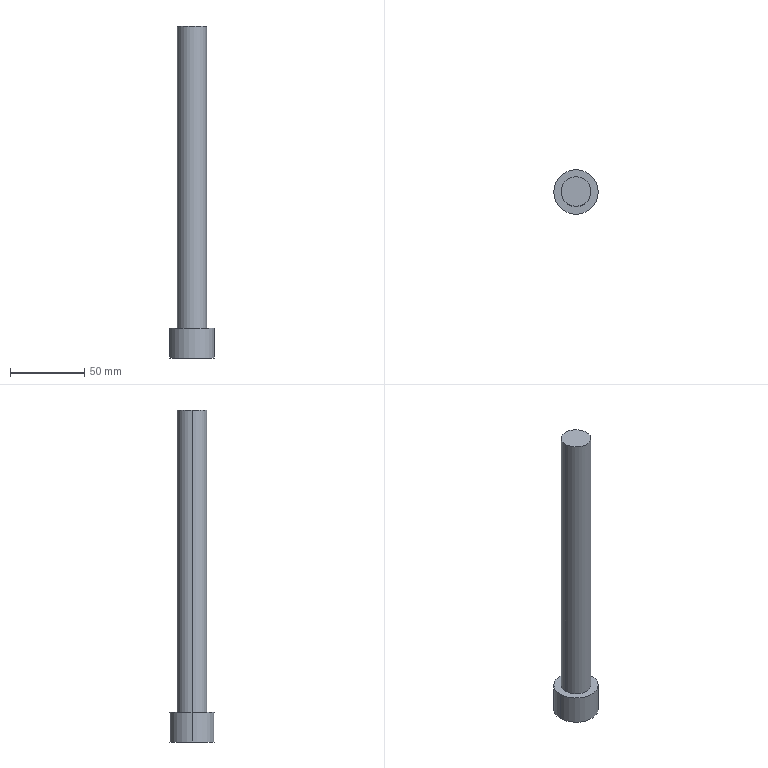Part | Creo | 1 solid | 14 faces | box 30 x 30 x 224 mm | volume 75420 mm3 | plane 10 | cylinder 4 | commonest cylinder face diameters 20 x2 30 x2
STEP:
#1=CARTESIAN_POINT('',(-235.,225.,-334.5));
#2=VERTEX_POINT('',#1);
#3=CARTESIAN_POINT('',(-265.,225.,-334.5));
#4=VERTEX_POINT('',#3);
#5=CARTESIAN_POINT('',(-250.,225.,-334.5));
#6=DIRECTION('',(0.,0.,-1.));
#7=DIRECTION('',(1.,0.,0.));
#8=AXIS2_PLACEMENT_3D('',#5,#6,#7);
#9=CIRCLE('',#8,15.);
#10=EDGE_CURVE('',#2,#4,#9,.T.);
#11=ORIENTED_EDGE('',*,*,#10,.F.);
#12=CARTESIAN_POINT('',(-250.,225.,-334.5));
#13=DIRECTION('',(0.,0.,-1.));
#14=DIRECTION('',(-1.,0.,0.));
#15=AXIS2_PLACEMENT_3D('',#12,#13,#14);
#16=CIRCLE('',#15,15.);
#17=EDGE_CURVE('',#4,#2,#16,.T.);
#18=ORIENTED_EDGE('',*,*,#17,.F.);
#19=EDGE_LOOP('',(#11,#18));
#20=FACE_OUTER_BOUND('',#19,.F.);
#21=CARTESIAN_POINT('',(-259.,219.804,-334.5));
#22=VERTEX_POINT('',#21);
#23=CARTESIAN_POINT('',(-250.,214.608,-334.5));
#24=VERTEX_POINT('',#23);
#25=CARTESIAN_POINT('',(-259.,219.804,-334.5));
#26=DIRECTION('',(0.866,-0.5,0.));
#27=VECTOR('',#26,10.392);
#28=LINE('',#25,#27);
#29=EDGE_CURVE('',#22,#24,#28,.T.);
#30=ORIENTED_EDGE('',*,*,#29,.F.);
#31=CARTESIAN_POINT('',(-259.,230.196,-334.5));
#32=VERTEX_POINT('',#31);
#33=CARTESIAN_POINT('',(-259.,219.804,-334.5));
#34=DIRECTION('',(0.,1.,0.));
#35=VECTOR('',#34,10.392);
#36=LINE('',#33,#35);
#37=EDGE_CURVE('',#22,#32,#36,.T.);
#38=ORIENTED_EDGE('',*,*,#37,.T.);
#39=CARTESIAN_POINT('',(-250.,235.392,-334.5));
#40=VERTEX_POINT('',#39);
#41=CARTESIAN_POINT('',(-250.,235.392,-334.5));
#42=DIRECTION('',(-0.866,-0.5,0.));
#43=VECTOR('',#42,10.392);
#44=LINE('',#41,#43);
#45=EDGE_CURVE('',#40,#32,#44,.T.);
#46=ORIENTED_EDGE('',*,*,#45,.F.);
#47=CARTESIAN_POINT('',(-241.,230.196,-334.5));
#48=VERTEX_POINT('',#47);
#49=CARTESIAN_POINT('',(-241.,230.196,-334.5));
#50=DIRECTION('',(-0.866,0.5,0.));
#51=VECTOR('',#50,10.392);
#52=LINE('',#49,#51);
#53=EDGE_CURVE('',#48,#40,#52,.T.);
#54=ORIENTED_EDGE('',*,*,#53,.F.);
#55=CARTESIAN_POINT('',(-241.,219.804,-334.5));
#56=VERTEX_POINT('',#55);
#57=CARTESIAN_POINT('',(-241.,230.196,-334.5));
#58=DIRECTION('',(0.,-1.,0.));
#59=VECTOR('',#58,10.392);
#60=LINE('',#57,#59);
#61=EDGE_CURVE('',#48,#56,#60,.T.);
#62=ORIENTED_EDGE('',*,*,#61,.T.);
#63=CARTESIAN_POINT('',(-250.,214.608,-334.5));
#64=DIRECTION('',(0.866,0.5,0.));
#65=VECTOR('',#64,10.392);
#66=LINE('',#63,#65);
#67=EDGE_CURVE('',#24,#56,#66,.T.);
#68=ORIENTED_EDGE('',*,*,#67,.F.);
#69=EDGE_LOOP('',(#30,#38,#46,#54,#62,#68));
#70=FACE_BOUND('',#69,.F.);
#71=CARTESIAN_POINT('',(-250.,225.,-334.5));
#72=DIRECTION('',(0.,0.,-1.));
#73=DIRECTION('',(-1.,0.,0.));
#74=AXIS2_PLACEMENT_3D('',#71,#72,#73);
#75=PLANE('',#74);
#76=ADVANCED_FACE('',(#20,#70),#75,.T.);
#77=CARTESIAN_POINT('',(-265.,225.,-314.5));
#78=VERTEX_POINT('',#77);
#79=CARTESIAN_POINT('',(-235.,225.,-314.5));
#80=VERTEX_POINT('',#79);
#81=CARTESIAN_POINT('',(-250.,225.,-314.5));
#82=DIRECTION('',(0.,0.,1.));
#83=DIRECTION('',(-1.,0.,0.));
#84=AXIS2_PLACEMENT_3D('',#81,#82,#83);
#85=CIRCLE('',#84,15.);
#86=EDGE_CURVE('',#78,#80,#85,.T.);
#87=ORIENTED_EDGE('',*,*,#86,.T.);
#88=CARTESIAN_POINT('',(-235.,225.,-334.5));
#89=DIRECTION('',(0.,0.,1.));
#90=VECTOR('',#89,20.);
#91=LINE('',#88,#90);
#92=EDGE_CURVE('',#2,#80,#91,.T.);
#93=ORIENTED_EDGE('',*,*,#92,.F.);
#94=ORIENTED_EDGE('',*,*,#10,.T.);
#95=CARTESIAN_POINT('',(-265.,225.,-334.5));
#96=DIRECTION('',(0.,0.,1.));
#97=VECTOR('',#96,20.);
#98=LINE('',#95,#97);
#99=EDGE_CURVE('',#4,#78,#98,.T.);
#100=ORIENTED_EDGE('',*,*,#99,.T.);
#101=EDGE_LOOP('',(#87,#93,#94,#100));
#102=FACE_OUTER_BOUND('',#101,.F.);
#103=CARTESIAN_POINT('',(-250.,225.,-334.5));
#104=DIRECTION('',(0.,0.,1.));
#105=DIRECTION('',(1.,0.,0.));
#106=AXIS2_PLACEMENT_3D('',#103,#104,#105);
#107=CYLINDRICAL_SURFACE('',#106,15.);
#108=ADVANCED_FACE('',(#102),#107,.T.);
#109=ORIENTED_EDGE('',*,*,#86,.F.);
#110=CARTESIAN_POINT('',(-250.,225.,-314.5));
#111=DIRECTION('',(0.,0.,1.));
#112=DIRECTION('',(1.,0.,0.));
#113=AXIS2_PLACEMENT_3D('',#110,#111,#112);
#114=CIRCLE('',#113,15.);
#115=EDGE_CURVE('',#80,#78,#114,.T.);
#116=ORIENTED_EDGE('',*,*,#115,.F.);
#117=EDGE_LOOP('',(#109,#116));
#118=FACE_OUTER_BOUND('',#117,.F.);
#119=CARTESIAN_POINT('',(-240.,225.,-314.5));
#120=VERTEX_POINT('',#119);
#121=CARTESIAN_POINT('',(-260.,225.,-314.5));
#122=VERTEX_POINT('',#121);
#123=CARTESIAN_POINT('',(-250.,225.,-314.5));
#124=DIRECTION('',(0.,0.,-1.));
#125=DIRECTION('',(1.,0.,0.));
#126=AXIS2_PLACEMENT_3D('',#123,#124,#125);
#127=CIRCLE('',#126,10.);
#128=EDGE_CURVE('',#120,#122,#127,.T.);
#129=ORIENTED_EDGE('',*,*,#128,.F.);
#130=CARTESIAN_POINT('',(-250.,225.,-314.5));
#131=DIRECTION('',(0.,0.,-1.));
#132=DIRECTION('',(-1.,0.,0.));
#133=AXIS2_PLACEMENT_3D('',#130,#131,#132);
#134=CIRCLE('',#133,10.);
#135=EDGE_CURVE('',#122,#120,#134,.T.);
#136=ORIENTED_EDGE('',*,*,#135,.F.);
#137=EDGE_LOOP('',(#129,#136));
#138=FACE_BOUND('',#137,.F.);
#139=CARTESIAN_POINT('',(-250.,225.,-314.5));
#140=DIRECTION('',(0.,0.,1.));
#141=DIRECTION('',(1.,0.,0.));
#142=AXIS2_PLACEMENT_3D('',#139,#140,#141);
#143=PLANE('',#142);
#144=ADVANCED_FACE('',(#118,#138),#143,.T.);
#145=ORIENTED_EDGE('',*,*,#128,.T.);
#146=CARTESIAN_POINT('',(-260.,225.,-110.5));
#147=VERTEX_POINT('',#146);
#148=CARTESIAN_POINT('',(-260.,225.,-314.5));
#149=DIRECTION('',(0.,0.,1.));
#150=VECTOR('',#149,204.);
#151=LINE('',#148,#150);
#152=EDGE_CURVE('',#122,#147,#151,.T.);
#153=ORIENTED_EDGE('',*,*,#152,.T.);
#154=CARTESIAN_POINT('',(-240.,225.,-110.5));
#155=VERTEX_POINT('',#154);
#156=CARTESIAN_POINT('',(-250.,225.,-110.5));
#157=DIRECTION('',(0.,0.,1.));
#158=DIRECTION('',(-1.,0.,0.));
#159=AXIS2_PLACEMENT_3D('',#156,#157,#158);
#160=CIRCLE('',#159,10.);
#161=EDGE_CURVE('',#147,#155,#160,.T.);
#162=ORIENTED_EDGE('',*,*,#161,.T.);
#163=CARTESIAN_POINT('',(-240.,225.,-314.5));
#164=DIRECTION('',(0.,0.,1.));
#165=VECTOR('',#164,204.);
#166=LINE('',#163,#165);
#167=EDGE_CURVE('',#120,#155,#166,.T.);
#168=ORIENTED_EDGE('',*,*,#167,.F.);
#169=EDGE_LOOP('',(#145,#153,#162,#168));
#170=FACE_OUTER_BOUND('',#169,.F.);
#171=CARTESIAN_POINT('',(-250.,225.,-334.5));
#172=DIRECTION('',(0.,0.,1.));
#173=DIRECTION('',(1.,0.,0.));
#174=AXIS2_PLACEMENT_3D('',#171,#172,#173);
#175=CYLINDRICAL_SURFACE('',#174,10.);
#176=ADVANCED_FACE('',(#170),#175,.T.);
#177=ORIENTED_EDGE('',*,*,#135,.T.);
#178=ORIENTED_EDGE('',*,*,#167,.T.);
#179=CARTESIAN_POINT('',(-250.,225.,-110.5));
#180=DIRECTION('',(0.,0.,1.));
#181=DIRECTION('',(1.,0.,0.));
#182=AXIS2_PLACEMENT_3D('',#179,#180,#181);
#183=CIRCLE('',#182,10.);
#184=EDGE_CURVE('',#155,#147,#183,.T.);
#185=ORIENTED_EDGE('',*,*,#184,.T.);
#186=ORIENTED_EDGE('',*,*,#152,.F.);
#187=EDGE_LOOP('',(#177,#178,#185,#186));
#188=FACE_OUTER_BOUND('',#187,.F.);
#189=CARTESIAN_POINT('',(-250.,225.,-334.5));
#190=DIRECTION('',(0.,0.,1.));
#191=DIRECTION('',(1.,0.,0.));
#192=AXIS2_PLACEMENT_3D('',#189,#190,#191);
#193=CYLINDRICAL_SURFACE('',#192,10.);
#194=ADVANCED_FACE('',(#188),#193,.T.);
#195=ORIENTED_EDGE('',*,*,#161,.F.);
#196=ORIENTED_EDGE('',*,*,#184,.F.);
#197=EDGE_LOOP('',(#195,#196));
#198=FACE_OUTER_BOUND('',#197,.F.);
#199=CARTESIAN_POINT('',(-250.,225.,-110.5));
#200=DIRECTION('',(0.,0.,1.));
#201=DIRECTION('',(1.,0.,0.));
#202=AXIS2_PLACEMENT_3D('',#199,#200,#201);
#203=PLANE('',#202);
#204=ADVANCED_FACE('',(#198),#203,.T.);
#205=ORIENTED_EDGE('',*,*,#115,.T.);
#206=ORIENTED_EDGE('',*,*,#99,.F.);
#207=ORIENTED_EDGE('',*,*,#17,.T.);
#208=ORIENTED_EDGE('',*,*,#92,.T.);
#209=EDGE_LOOP('',(#205,#206,#207,#208));
#210=FACE_OUTER_BOUND('',#209,.F.);
#211=CARTESIAN_POINT('',(-250.,225.,-334.5));
#212=DIRECTION('',(0.,0.,1.));
#213=DIRECTION('',(1.,0.,0.));
#214=AXIS2_PLACEMENT_3D('',#211,#212,#213);
#215=CYLINDRICAL_SURFACE('',#214,15.);
#216=ADVANCED_FACE('',(#210),#215,.T.);
#217=CARTESIAN_POINT('',(-250.,214.608,-324.5));
#218=VERTEX_POINT('',#217);
#219=CARTESIAN_POINT('',(-259.,219.804,-324.5));
#220=VERTEX_POINT('',#219);
#221=CARTESIAN_POINT('',(-250.,214.608,-324.5));
#222=DIRECTION('',(-0.866,0.5,0.));
#223=VECTOR('',#222,10.392);
#224=LINE('',#221,#223);
#225=EDGE_CURVE('',#218,#220,#224,.T.);
#226=ORIENTED_EDGE('',*,*,#225,.T.);
#227=CARTESIAN_POINT('',(-259.,219.804,-324.5));
#228=DIRECTION('',(0.,0.,-1.));
#229=VECTOR('',#228,10.);
#230=LINE('',#227,#229);
#231=EDGE_CURVE('',#220,#22,#230,.T.);
#232=ORIENTED_EDGE('',*,*,#231,.T.);
#233=ORIENTED_EDGE('',*,*,#29,.T.);
#234=CARTESIAN_POINT('',(-250.,214.608,-324.5));
#235=DIRECTION('',(0.,0.,-1.));
#236=VECTOR('',#235,10.);
#237=LINE('',#234,#236);
#238=EDGE_CURVE('',#218,#24,#237,.T.);
#239=ORIENTED_EDGE('',*,*,#238,.F.);
#240=EDGE_LOOP('',(#226,#232,#233,#239));
#241=FACE_OUTER_BOUND('',#240,.F.);
#242=CARTESIAN_POINT('',(-254.5,217.206,-329.5));
#243=DIRECTION('',(-0.5,-0.866,0.));
#244=DIRECTION('',(0.866,-0.5,0.));
#245=AXIS2_PLACEMENT_3D('',#242,#243,#244);
#246=PLANE('',#245);
#247=ADVANCED_FACE('',(#241),#246,.F.);
#248=CARTESIAN_POINT('',(-259.,230.196,-324.5));
#249=VERTEX_POINT('',#248);
#250=CARTESIAN_POINT('',(-259.,219.804,-324.5));
#251=DIRECTION('',(0.,1.,0.));
#252=VECTOR('',#251,10.392);
#253=LINE('',#250,#252);
#254=EDGE_CURVE('',#220,#249,#253,.T.);
#255=ORIENTED_EDGE('',*,*,#254,.F.);
#256=ORIENTED_EDGE('',*,*,#225,.F.);
#257=CARTESIAN_POINT('',(-241.,219.804,-324.5));
#258=VERTEX_POINT('',#257);
#259=CARTESIAN_POINT('',(-241.,219.804,-324.5));
#260=DIRECTION('',(-0.866,-0.5,0.));
#261=VECTOR('',#260,10.392);
#262=LINE('',#259,#261);
#263=EDGE_CURVE('',#258,#218,#262,.T.);
#264=ORIENTED_EDGE('',*,*,#263,.F.);
#265=CARTESIAN_POINT('',(-241.,230.196,-324.5));
#266=VERTEX_POINT('',#265);
#267=CARTESIAN_POINT('',(-241.,230.196,-324.5));
#268=DIRECTION('',(0.,-1.,0.));
#269=VECTOR('',#268,10.392);
#270=LINE('',#267,#269);
#271=EDGE_CURVE('',#266,#258,#270,.T.);
#272=ORIENTED_EDGE('',*,*,#271,.F.);
#273=CARTESIAN_POINT('',(-250.,235.392,-324.5));
#274=VERTEX_POINT('',#273);
#275=CARTESIAN_POINT('',(-250.,235.392,-324.5));
#276=DIRECTION('',(0.866,-0.5,0.));
#277=VECTOR('',#276,10.392);
#278=LINE('',#275,#277);
#279=EDGE_CURVE('',#274,#266,#278,.T.);
#280=ORIENTED_EDGE('',*,*,#279,.F.);
#281=CARTESIAN_POINT('',(-259.,230.196,-324.5));
#282=DIRECTION('',(0.866,0.5,0.));
#283=VECTOR('',#282,10.392);
#284=LINE('',#281,#283);
#285=EDGE_CURVE('',#249,#274,#284,.T.);
#286=ORIENTED_EDGE('',*,*,#285,.F.);
#287=EDGE_LOOP('',(#255,#256,#264,#272,#280,#286));
#288=FACE_OUTER_BOUND('',#287,.F.);
#289=CARTESIAN_POINT('',(-250.,225.,-324.5));
#290=DIRECTION('',(0.,0.,1.));
#291=DIRECTION('',(1.,0.,0.));
#292=AXIS2_PLACEMENT_3D('',#289,#290,#291);
#293=PLANE('',#292);
#294=ADVANCED_FACE('',(#288),#293,.F.);
#295=ORIENTED_EDGE('',*,*,#254,.T.);
#296=CARTESIAN_POINT('',(-259.,230.196,-324.5));
#297=DIRECTION('',(0.,0.,-1.));
#298=VECTOR('',#297,10.);
#299=LINE('',#296,#298);
#300=EDGE_CURVE('',#249,#32,#299,.T.);
#301=ORIENTED_EDGE('',*,*,#300,.T.);
#302=ORIENTED_EDGE('',*,*,#37,.F.);
#303=ORIENTED_EDGE('',*,*,#231,.F.);
#304=EDGE_LOOP('',(#295,#301,#302,#303));
#305=FACE_OUTER_BOUND('',#304,.F.);
#306=CARTESIAN_POINT('',(-259.,225.,-329.5));
#307=DIRECTION('',(-1.,0.,0.));
#308=DIRECTION('',(0.,0.,1.));
#309=AXIS2_PLACEMENT_3D('',#306,#307,#308);
#310=PLANE('',#309);
#311=ADVANCED_FACE('',(#305),#310,.F.);
#312=ORIENTED_EDGE('',*,*,#285,.T.);
#313=CARTESIAN_POINT('',(-250.,235.392,-324.5));
#314=DIRECTION('',(0.,0.,-1.));
#315=VECTOR('',#314,10.);
#316=LINE('',#313,#315);
#317=EDGE_CURVE('',#274,#40,#316,.T.);
#318=ORIENTED_EDGE('',*,*,#317,.T.);
#319=ORIENTED_EDGE('',*,*,#45,.T.);
#320=ORIENTED_EDGE('',*,*,#300,.F.);
#321=EDGE_LOOP('',(#312,#318,#319,#320));
#322=FACE_OUTER_BOUND('',#321,.F.);
#323=CARTESIAN_POINT('',(-254.5,232.794,-329.5));
#324=DIRECTION('',(-0.5,0.866,0.));
#325=DIRECTION('',(-0.866,-0.5,0.));
#326=AXIS2_PLACEMENT_3D('',#323,#324,#325);
#327=PLANE('',#326);
#328=ADVANCED_FACE('',(#322),#327,.F.);
#329=ORIENTED_EDGE('',*,*,#279,.T.);
#330=CARTESIAN_POINT('',(-241.,230.196,-324.5));
#331=DIRECTION('',(0.,0.,-1.));
#332=VECTOR('',#331,10.);
#333=LINE('',#330,#332);
#334=EDGE_CURVE('',#266,#48,#333,.T.);
#335=ORIENTED_EDGE('',*,*,#334,.T.);
#336=ORIENTED_EDGE('',*,*,#53,.T.);
#337=ORIENTED_EDGE('',*,*,#317,.F.);
#338=EDGE_LOOP('',(#329,#335,#336,#337));
#339=FACE_OUTER_BOUND('',#338,.F.);
#340=CARTESIAN_POINT('',(-245.5,232.794,-329.5));
#341=DIRECTION('',(0.5,0.866,0.));
#342=DIRECTION('',(-0.866,0.5,0.));
#343=AXIS2_PLACEMENT_3D('',#340,#341,#342);
#344=PLANE('',#343);
#345=ADVANCED_FACE('',(#339),#344,.F.);
#346=ORIENTED_EDGE('',*,*,#271,.T.);
#347=CARTESIAN_POINT('',(-241.,219.804,-324.5));
#348=DIRECTION('',(0.,0.,-1.));
#349=VECTOR('',#348,10.);
#350=LINE('',#347,#349);
#351=EDGE_CURVE('',#258,#56,#350,.T.);
#352=ORIENTED_EDGE('',*,*,#351,.T.);
#353=ORIENTED_EDGE('',*,*,#61,.F.);
#354=ORIENTED_EDGE('',*,*,#334,.F.);
#355=EDGE_LOOP('',(#346,#352,#353,#354));
#356=FACE_OUTER_BOUND('',#355,.F.);
#357=CARTESIAN_POINT('',(-241.,225.,-329.5));
#358=DIRECTION('',(1.,0.,0.));
#359=DIRECTION('',(0.,0.,-1.));
#360=AXIS2_PLACEMENT_3D('',#357,#358,#359);
#361=PLANE('',#360);
#362=ADVANCED_FACE('',(#356),#361,.F.);
#363=ORIENTED_EDGE('',*,*,#263,.T.);
#364=ORIENTED_EDGE('',*,*,#238,.T.);
#365=ORIENTED_EDGE('',*,*,#67,.T.);
#366=ORIENTED_EDGE('',*,*,#351,.F.);
#367=EDGE_LOOP('',(#363,#364,#365,#366));
#368=FACE_OUTER_BOUND('',#367,.F.);
#369=CARTESIAN_POINT('',(-245.5,217.206,-329.5));
#370=DIRECTION('',(0.5,-0.866,0.));
#371=DIRECTION('',(0.866,0.5,0.));
#372=AXIS2_PLACEMENT_3D('',#369,#370,#371);
#373=PLANE('',#372);
#374=ADVANCED_FACE('',(#368),#373,.F.);
#375=CLOSED_SHELL('',(#76,#108,#144,#176,#194,#204,#216,#247,#294,#311,#328,#345,#362,#374));
#376=MANIFOLD_SOLID_BREP('',#375);
#377=(LENGTH_UNIT()NAMED_UNIT(*)SI_UNIT(.MILLI.,.METRE.));
#378=UNCERTAINTY_MEASURE_WITH_UNIT(LENGTH_MEASURE(0.0228),#377,'','');
#379=(NAMED_UNIT(*)PLANE_ANGLE_UNIT()SI_UNIT($,.RADIAN.));
#380=PLANE_ANGLE_MEASURE_WITH_UNIT(PLANE_ANGLE_MEASURE(0.01745),#379);
#381=(CONVERSION_BASED_UNIT('DEGREE',#380)NAMED_UNIT(*)PLANE_ANGLE_UNIT());
#382=(NAMED_UNIT(*)SI_UNIT($,.STERADIAN.)SOLID_ANGLE_UNIT());
#383=(GEOMETRIC_REPRESENTATION_CONTEXT(3)GLOBAL_UNCERTAINTY_ASSIGNED_CONTEXT((#378))GLOBAL_UNIT_ASSIGNED_CONTEXT((#377,#381,#382))REPRESENTATION_CONTEXT('',''));
#384=ADVANCED_BREP_SHAPE_REPRESENTATION('',(#376),#383);